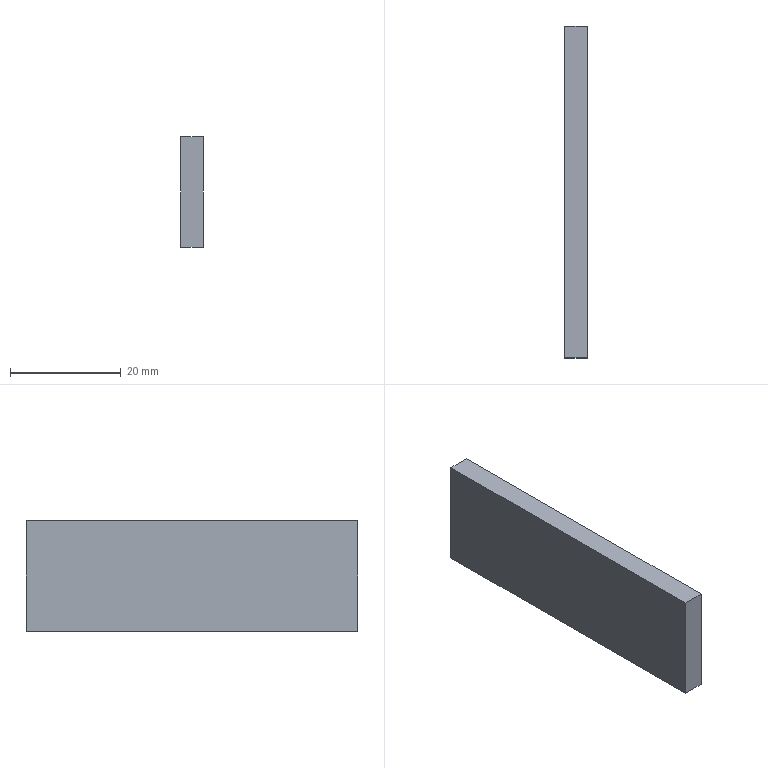Part | SolidWorks | features Extrusion 1 | 1 solid | 6 faces | box 4 x 60 x 20 mm | volume 4800 mm3 | plane 6
STEP:
#1=CARTESIAN_POINT('',(0.,60.,0.));
#2=VERTEX_POINT('',#1);
#3=CARTESIAN_POINT('',(0.,0.,0.));
#4=VERTEX_POINT('',#3);
#5=CARTESIAN_POINT('',(0.,0.,0.));
#6=DIRECTION('',(0.,-1.,0.));
#7=VECTOR('',#6,1000.);
#8=LINE('',#5,#7);
#9=EDGE_CURVE('',#2,#4,#8,.T.);
#10=ORIENTED_EDGE('',*,*,#9,.T.);
#11=CARTESIAN_POINT('',(4.,0.,0.));
#12=VERTEX_POINT('',#11);
#13=CARTESIAN_POINT('',(4.,0.,0.));
#14=DIRECTION('',(-1.,0.,0.));
#15=VECTOR('',#14,1000.);
#16=LINE('',#13,#15);
#17=EDGE_CURVE('',#12,#4,#16,.T.);
#18=ORIENTED_EDGE('',*,*,#17,.F.);
#19=CARTESIAN_POINT('',(4.,60.,0.));
#20=VERTEX_POINT('',#19);
#21=CARTESIAN_POINT('',(4.,0.,0.));
#22=DIRECTION('',(0.,-1.,0.));
#23=VECTOR('',#22,1000.);
#24=LINE('',#21,#23);
#25=EDGE_CURVE('',#20,#12,#24,.T.);
#26=ORIENTED_EDGE('',*,*,#25,.F.);
#27=CARTESIAN_POINT('',(4.,60.,0.));
#28=DIRECTION('',(-1.,0.,0.));
#29=VECTOR('',#28,1000.);
#30=LINE('',#27,#29);
#31=EDGE_CURVE('',#20,#2,#30,.T.);
#32=ORIENTED_EDGE('',*,*,#31,.T.);
#33=EDGE_LOOP('',(#10,#18,#26,#32));
#34=FACE_OUTER_BOUND('',#33,.T.);
#35=CARTESIAN_POINT('',(4.,0.,0.));
#36=DIRECTION('',(0.,0.,-1.));
#37=DIRECTION('',(-1.,0.,0.));
#38=AXIS2_PLACEMENT_3D('',#35,#36,#37);
#39=PLANE('',#38);
#40=ADVANCED_FACE('',(#34),#39,.F.);
#41=CARTESIAN_POINT('',(0.,0.,-20.));
#42=VERTEX_POINT('',#41);
#43=CARTESIAN_POINT('',(0.,0.,0.));
#44=DIRECTION('',(0.,0.,-1.));
#45=VECTOR('',#44,1000.);
#46=LINE('',#43,#45);
#47=EDGE_CURVE('',#4,#42,#46,.T.);
#48=ORIENTED_EDGE('',*,*,#47,.T.);
#49=CARTESIAN_POINT('',(4.,0.,-20.));
#50=VERTEX_POINT('',#49);
#51=CARTESIAN_POINT('',(4.,0.,-20.));
#52=DIRECTION('',(-1.,0.,0.));
#53=VECTOR('',#52,1000.);
#54=LINE('',#51,#53);
#55=EDGE_CURVE('',#50,#42,#54,.T.);
#56=ORIENTED_EDGE('',*,*,#55,.F.);
#57=CARTESIAN_POINT('',(4.,0.,0.));
#58=DIRECTION('',(0.,0.,-1.));
#59=VECTOR('',#58,1000.);
#60=LINE('',#57,#59);
#61=EDGE_CURVE('',#12,#50,#60,.T.);
#62=ORIENTED_EDGE('',*,*,#61,.F.);
#63=ORIENTED_EDGE('',*,*,#17,.T.);
#64=EDGE_LOOP('',(#48,#56,#62,#63));
#65=FACE_OUTER_BOUND('',#64,.T.);
#66=CARTESIAN_POINT('',(4.,0.,0.));
#67=DIRECTION('',(0.,1.,0.));
#68=DIRECTION('',(0.,0.,1.));
#69=AXIS2_PLACEMENT_3D('',#66,#67,#68);
#70=PLANE('',#69);
#71=ADVANCED_FACE('',(#65),#70,.F.);
#72=CARTESIAN_POINT('',(0.,60.,-20.));
#73=VERTEX_POINT('',#72);
#74=CARTESIAN_POINT('',(0.,0.,-20.));
#75=DIRECTION('',(0.,1.,0.));
#76=VECTOR('',#75,1000.);
#77=LINE('',#74,#76);
#78=EDGE_CURVE('',#42,#73,#77,.T.);
#79=ORIENTED_EDGE('',*,*,#78,.T.);
#80=CARTESIAN_POINT('',(4.,60.,-20.));
#81=VERTEX_POINT('',#80);
#82=CARTESIAN_POINT('',(4.,60.,-20.));
#83=DIRECTION('',(-1.,0.,0.));
#84=VECTOR('',#83,1000.);
#85=LINE('',#82,#84);
#86=EDGE_CURVE('',#81,#73,#85,.T.);
#87=ORIENTED_EDGE('',*,*,#86,.F.);
#88=CARTESIAN_POINT('',(4.,0.,-20.));
#89=DIRECTION('',(0.,1.,0.));
#90=VECTOR('',#89,1000.);
#91=LINE('',#88,#90);
#92=EDGE_CURVE('',#50,#81,#91,.T.);
#93=ORIENTED_EDGE('',*,*,#92,.F.);
#94=ORIENTED_EDGE('',*,*,#55,.T.);
#95=EDGE_LOOP('',(#79,#87,#93,#94));
#96=FACE_OUTER_BOUND('',#95,.T.);
#97=CARTESIAN_POINT('',(4.,0.,-20.));
#98=DIRECTION('',(0.,0.,1.));
#99=DIRECTION('',(1.,0.,0.));
#100=AXIS2_PLACEMENT_3D('',#97,#98,#99);
#101=PLANE('',#100);
#102=ADVANCED_FACE('',(#96),#101,.F.);
#103=CARTESIAN_POINT('',(0.,60.,0.));
#104=DIRECTION('',(0.,0.,1.));
#105=VECTOR('',#104,1000.);
#106=LINE('',#103,#105);
#107=EDGE_CURVE('',#73,#2,#106,.T.);
#108=ORIENTED_EDGE('',*,*,#107,.T.);
#109=ORIENTED_EDGE('',*,*,#31,.F.);
#110=CARTESIAN_POINT('',(4.,60.,0.));
#111=DIRECTION('',(0.,0.,1.));
#112=VECTOR('',#111,1000.);
#113=LINE('',#110,#112);
#114=EDGE_CURVE('',#81,#20,#113,.T.);
#115=ORIENTED_EDGE('',*,*,#114,.F.);
#116=ORIENTED_EDGE('',*,*,#86,.T.);
#117=EDGE_LOOP('',(#108,#109,#115,#116));
#118=FACE_OUTER_BOUND('',#117,.T.);
#119=CARTESIAN_POINT('',(4.,60.,0.));
#120=DIRECTION('',(0.,-1.,0.));
#121=DIRECTION('',(0.,0.,-1.));
#122=AXIS2_PLACEMENT_3D('',#119,#120,#121);
#123=PLANE('',#122);
#124=ADVANCED_FACE('',(#118),#123,.F.);
#125=ORIENTED_EDGE('',*,*,#25,.T.);
#126=ORIENTED_EDGE('',*,*,#61,.T.);
#127=ORIENTED_EDGE('',*,*,#92,.T.);
#128=ORIENTED_EDGE('',*,*,#114,.T.);
#129=EDGE_LOOP('',(#125,#126,#127,#128));
#130=FACE_OUTER_BOUND('',#129,.T.);
#131=CARTESIAN_POINT('',(4.,0.,0.));
#132=DIRECTION('',(-1.,0.,0.));
#133=DIRECTION('',(0.,0.,1.));
#134=AXIS2_PLACEMENT_3D('',#131,#132,#133);
#135=PLANE('',#134);
#136=ADVANCED_FACE('',(#130),#135,.F.);
#137=ORIENTED_EDGE('',*,*,#9,.F.);
#138=ORIENTED_EDGE('',*,*,#107,.F.);
#139=ORIENTED_EDGE('',*,*,#78,.F.);
#140=ORIENTED_EDGE('',*,*,#47,.F.);
#141=EDGE_LOOP('',(#137,#138,#139,#140));
#142=FACE_OUTER_BOUND('',#141,.T.);
#143=CARTESIAN_POINT('',(0.,0.,0.));
#144=DIRECTION('',(-1.,0.,0.));
#145=DIRECTION('',(0.,0.,1.));
#146=AXIS2_PLACEMENT_3D('',#143,#144,#145);
#147=PLANE('',#146);
#148=ADVANCED_FACE('',(#142),#147,.T.);
#149=CLOSED_SHELL('',(#40,#71,#102,#124,#136,#148));
#150=MANIFOLD_SOLID_BREP('',#149);
#151=CARTESIAN_POINT('',(0.,0.,0.));
#152=DIRECTION('',(0.,0.,1.));
#153=DIRECTION('',(1.,0.,0.));
#154=AXIS2_PLACEMENT_3D('',#151,#152,#153);
#155=(LENGTH_UNIT()NAMED_UNIT(*)SI_UNIT(.MILLI.,.METRE.));
#156=UNCERTAINTY_MEASURE_WITH_UNIT(LENGTH_MEASURE(0.00001),#155,'','');
#157=(NAMED_UNIT(*)PLANE_ANGLE_UNIT()SI_UNIT($,.RADIAN.));
#158=(NAMED_UNIT(*)SI_UNIT($,.STERADIAN.)SOLID_ANGLE_UNIT());
#159=(GEOMETRIC_REPRESENTATION_CONTEXT(3)GLOBAL_UNCERTAINTY_ASSIGNED_CONTEXT((#156))GLOBAL_UNIT_ASSIGNED_CONTEXT((#155,#157,#158))REPRESENTATION_CONTEXT('',''));
#160=ADVANCED_BREP_SHAPE_REPRESENTATION('',(#150,#154),#159);